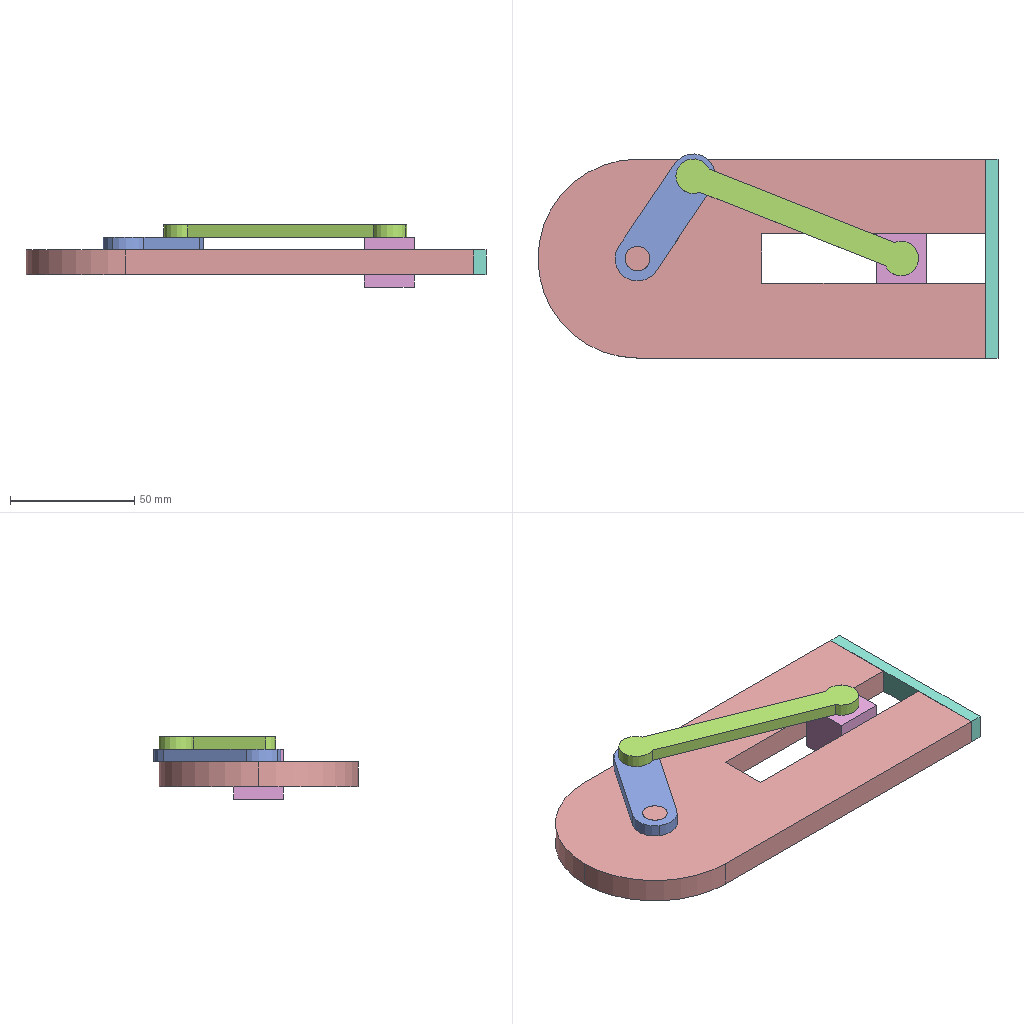Assembly | SolidWorks | 5 different items | 5 placed | box 185 x 82 x 25 mm
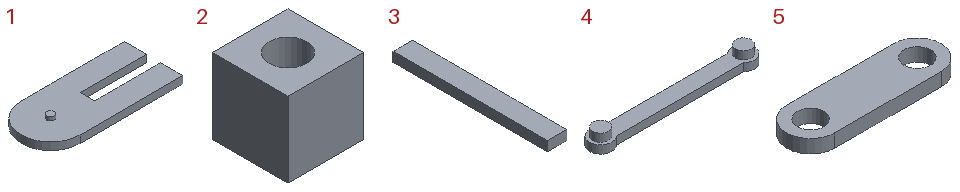Parts list (item | quantity | size | volume | features):
1 | x1 | 180 x 80 x 15 mm | 119525 mm3 | features Boss 1, Extrusion 1
2 | x1 | 20 x 20 x 20 mm | 6429 mm3 | features Cut 1, Extrusion 1
3 | x1 | 10 x 80 x 5 mm | 4000 mm3 | features Extrusion 1
4 | x1 | 104 x 14 x 10 mm | 6190 mm3 | features Boss 1, Extrusion 1
5 | x1 | 58 x 18 x 5 mm | 4087 mm3 | features Cut 1, Extrusion 1
Mates (type | each side: item.copy, entity, surface, feature):
Concentric | 1.1 face cylinder Boss-Extrude1 | 5.1 face cylinder Cut-Extrude1
Coincident | 1.1 face plane Base-Extrude | 5.1 face plane Base-Extrude
Concentric | 5.1 face cylinder Cut-Extrude1 | 4.1 face cylinder Boss-Extrude1
Coincident | 5.1 face plane Base-Extrude | 4.1 face plane Base-Extrude
Concentric | 4.1 face cylinder Boss-Extrude1 | 2.1 face cylinder Cut-Extrude1
Coincident | 4.1 face plane Base-Extrude | 2.1 face plane Base-Extrude
Coincident | 1.1 edge | 2.1 face plane Base-Extrude
Coincident | 1.1 face plane Base-Extrude | 3.1 face plane Base-Extrude | 3 times